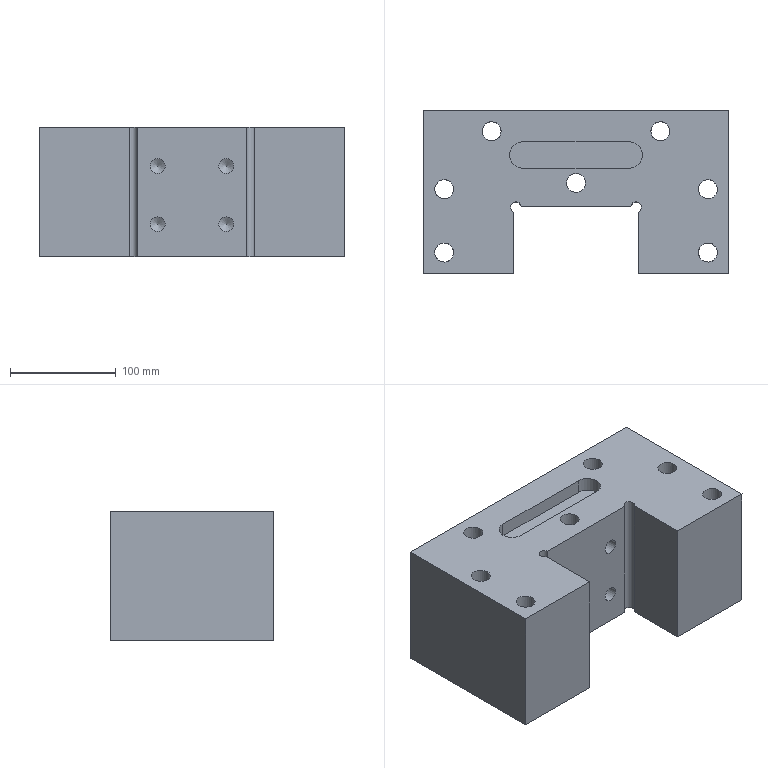Part | STEP file | lll_id778_x_t | 1 solid | 50 faces | box 290 x 155 x 123 mm | volume 4112201 mm3 | cylinder 24 | plane 20 | cone 6 | commonest cylinder face diameters 18.009 x7 26.007 x7 14 x6 10 x2 25 x2
STEP:
#1=CARTESIAN_POINT('',(2079.432,-574.,39.5));
#2=VERTEX_POINT('',#1);
#3=CARTESIAN_POINT('',(2092.435,-574.,39.5));
#4=DIRECTION('',(0.,0.,-1.));
#5=DIRECTION('',(-1.,0.,0.));
#6=AXIS2_PLACEMENT_3D('',#3,#4,#5);
#7=CIRCLE('',#6,13.004);
#8=EDGE_CURVE('',#2,#2,#7,.T.);
#9=ORIENTED_EDGE('',*,*,#8,.F.);
#10=EDGE_LOOP('',(#9));
#11=FACE_BOUND('',#10,.T.);
#12=CARTESIAN_POINT('',(1980.439,-640.,39.5));
#13=VERTEX_POINT('',#12);
#14=CARTESIAN_POINT('',(1967.435,-640.,39.5));
#15=DIRECTION('',(0.,0.,-1.));
#16=DIRECTION('',(1.,0.,0.));
#17=AXIS2_PLACEMENT_3D('',#14,#15,#16);
#18=CIRCLE('',#17,13.004);
#19=EDGE_CURVE('',#13,#13,#18,.T.);
#20=ORIENTED_EDGE('',*,*,#19,.F.);
#21=EDGE_LOOP('',(#20));
#22=FACE_BOUND('',#21,.T.);
#23=CARTESIAN_POINT('',(2230.439,-640.,39.5));
#24=VERTEX_POINT('',#23);
#25=CARTESIAN_POINT('',(2217.435,-640.,39.5));
#26=DIRECTION('',(0.,0.,-1.));
#27=DIRECTION('',(1.,0.,0.));
#28=AXIS2_PLACEMENT_3D('',#25,#26,#27);
#29=CIRCLE('',#28,13.004);
#30=EDGE_CURVE('',#24,#24,#29,.T.);
#31=ORIENTED_EDGE('',*,*,#30,.F.);
#32=EDGE_LOOP('',(#31));
#33=FACE_BOUND('',#32,.T.);
#34=CARTESIAN_POINT('',(1947.435,-660.,39.5));
#35=VERTEX_POINT('',#34);
#36=CARTESIAN_POINT('',(1947.435,-505.,39.5));
#37=VERTEX_POINT('',#36);
#38=CARTESIAN_POINT('',(1947.435,-551.,39.5));
#39=DIRECTION('',(0.,1.,0.));
#40=VECTOR('',#39,1.);
#41=LINE('',#38,#40);
#42=EDGE_CURVE('',#35,#37,#41,.T.);
#43=ORIENTED_EDGE('',*,*,#42,.T.);
#44=CARTESIAN_POINT('',(2237.435,-505.,39.5));
#45=VERTEX_POINT('',#44);
#46=CARTESIAN_POINT('',(2172.935,-505.,39.5));
#47=DIRECTION('',(1.,0.,0.));
#48=VECTOR('',#47,1.);
#49=LINE('',#46,#48);
#50=EDGE_CURVE('',#37,#45,#49,.T.);
#51=ORIENTED_EDGE('',*,*,#50,.T.);
#52=CARTESIAN_POINT('',(2237.435,-660.,39.5));
#53=VERTEX_POINT('',#52);
#54=CARTESIAN_POINT('',(2237.435,-631.,39.5));
#55=DIRECTION('',(0.,-1.,0.));
#56=VECTOR('',#55,1.);
#57=LINE('',#54,#56);
#58=EDGE_CURVE('',#45,#53,#57,.T.);
#59=ORIENTED_EDGE('',*,*,#58,.T.);
#60=CARTESIAN_POINT('',(2151.435,-660.,39.5));
#61=VERTEX_POINT('',#60);
#62=CARTESIAN_POINT('',(2173.935,-660.,39.5));
#63=DIRECTION('',(-1.,0.,0.));
#64=VECTOR('',#63,1.);
#65=LINE('',#62,#64);
#66=EDGE_CURVE('',#53,#61,#65,.T.);
#67=ORIENTED_EDGE('',*,*,#66,.T.);
#68=CARTESIAN_POINT('',(2151.435,-601.583,39.5));
#69=VERTEX_POINT('',#68);
#70=CARTESIAN_POINT('',(2151.435,-574.,39.5));
#71=DIRECTION('',(0.,1.,0.));
#72=VECTOR('',#71,1.);
#73=LINE('',#70,#72);
#74=EDGE_CURVE('',#61,#69,#73,.T.);
#75=ORIENTED_EDGE('',*,*,#74,.T.);
#76=CARTESIAN_POINT('',(2144.536,-596.,39.5));
#77=VERTEX_POINT('',#76);
#78=CARTESIAN_POINT('',(2149.435,-597.,39.5));
#79=DIRECTION('',(0.,0.,1.));
#80=DIRECTION('',(-1.,0.,0.));
#81=AXIS2_PLACEMENT_3D('',#78,#79,#80);
#82=CIRCLE('',#81,5.);
#83=EDGE_CURVE('',#69,#77,#82,.T.);
#84=ORIENTED_EDGE('',*,*,#83,.T.);
#85=CARTESIAN_POINT('',(2040.334,-596.,39.5));
#86=VERTEX_POINT('',#85);
#87=CARTESIAN_POINT('',(2137.864,-596.,39.5));
#88=DIRECTION('',(-1.,0.,0.));
#89=VECTOR('',#88,1.);
#90=LINE('',#87,#89);
#91=EDGE_CURVE('',#77,#86,#90,.T.);
#92=ORIENTED_EDGE('',*,*,#91,.T.);
#93=CARTESIAN_POINT('',(2033.435,-601.583,39.5));
#94=VERTEX_POINT('',#93);
#95=CARTESIAN_POINT('',(2035.435,-597.,39.5));
#96=DIRECTION('',(0.,0.,-1.));
#97=DIRECTION('',(-1.,0.,0.));
#98=AXIS2_PLACEMENT_3D('',#95,#96,#97);
#99=CIRCLE('',#98,5.);
#100=EDGE_CURVE('',#94,#86,#99,.T.);
#101=ORIENTED_EDGE('',*,*,#100,.F.);
#102=CARTESIAN_POINT('',(2033.435,-660.,39.5));
#103=VERTEX_POINT('',#102);
#104=CARTESIAN_POINT('',(2033.435,-631.,39.5));
#105=DIRECTION('',(0.,-1.,0.));
#106=VECTOR('',#105,1.);
#107=LINE('',#104,#106);
#108=EDGE_CURVE('',#94,#103,#107,.T.);
#109=ORIENTED_EDGE('',*,*,#108,.T.);
#110=CARTESIAN_POINT('',(1972.935,-660.,39.5));
#111=DIRECTION('',(-1.,0.,0.));
#112=VECTOR('',#111,1.);
#113=LINE('',#110,#112);
#114=EDGE_CURVE('',#103,#35,#113,.T.);
#115=ORIENTED_EDGE('',*,*,#114,.T.);
#116=EDGE_LOOP('',(#43,#51,#59,#67,#75,#84,#92,#101,#109,#115));
#117=FACE_BOUND('',#116,.T.);
#118=CARTESIAN_POINT('',(1986.436,-603.999,39.5));
#119=VERTEX_POINT('',#118);
#120=CARTESIAN_POINT('',(1993.436,-603.999,39.5));
#121=DIRECTION('',(0.,0.,-1.));
#122=DIRECTION('',(-1.,0.,0.));
#123=AXIS2_PLACEMENT_3D('',#120,#121,#122);
#124=CIRCLE('',#123,7.);
#125=EDGE_CURVE('',#119,#119,#124,.T.);
#126=ORIENTED_EDGE('',*,*,#125,.F.);
#127=EDGE_LOOP('',(#126));
#128=FACE_BOUND('',#127,.T.);
#129=CARTESIAN_POINT('',(2184.434,-603.999,39.5));
#130=VERTEX_POINT('',#129);
#131=CARTESIAN_POINT('',(2191.434,-603.999,39.5));
#132=DIRECTION('',(0.,0.,-1.));
#133=DIRECTION('',(-1.,0.,0.));
#134=AXIS2_PLACEMENT_3D('',#131,#132,#133);
#135=CIRCLE('',#134,7.);
#136=EDGE_CURVE('',#130,#130,#135,.T.);
#137=ORIENTED_EDGE('',*,*,#136,.F.);
#138=EDGE_LOOP('',(#137));
#139=FACE_BOUND('',#138,.T.);
#140=CARTESIAN_POINT('',(2230.439,-580.,39.5));
#141=VERTEX_POINT('',#140);
#142=CARTESIAN_POINT('',(2217.435,-580.,39.5));
#143=DIRECTION('',(0.,0.,-1.));
#144=DIRECTION('',(1.,0.,0.));
#145=AXIS2_PLACEMENT_3D('',#142,#143,#144);
#146=CIRCLE('',#145,13.004);
#147=EDGE_CURVE('',#141,#141,#146,.T.);
#148=ORIENTED_EDGE('',*,*,#147,.F.);
#149=EDGE_LOOP('',(#148));
#150=FACE_BOUND('',#149,.T.);
#151=CARTESIAN_POINT('',(2185.439,-525.,39.5));
#152=VERTEX_POINT('',#151);
#153=CARTESIAN_POINT('',(2172.435,-525.,39.5));
#154=DIRECTION('',(0.,0.,-1.));
#155=DIRECTION('',(1.,0.,0.));
#156=AXIS2_PLACEMENT_3D('',#153,#154,#155);
#157=CIRCLE('',#156,13.004);
#158=EDGE_CURVE('',#152,#152,#157,.T.);
#159=ORIENTED_EDGE('',*,*,#158,.F.);
#160=EDGE_LOOP('',(#159));
#161=FACE_BOUND('',#160,.T.);
#162=CARTESIAN_POINT('',(1980.439,-580.,39.5));
#163=VERTEX_POINT('',#162);
#164=CARTESIAN_POINT('',(1967.435,-580.,39.5));
#165=DIRECTION('',(0.,0.,-1.));
#166=DIRECTION('',(1.,0.,0.));
#167=AXIS2_PLACEMENT_3D('',#164,#165,#166);
#168=CIRCLE('',#167,13.004);
#169=EDGE_CURVE('',#163,#163,#168,.T.);
#170=ORIENTED_EDGE('',*,*,#169,.F.);
#171=EDGE_LOOP('',(#170));
#172=FACE_BOUND('',#171,.T.);
#173=CARTESIAN_POINT('',(1999.432,-525.,39.5));
#174=VERTEX_POINT('',#173);
#175=CARTESIAN_POINT('',(2012.435,-525.,39.5));
#176=DIRECTION('',(0.,0.,1.));
#177=DIRECTION('',(-1.,0.,0.));
#178=AXIS2_PLACEMENT_3D('',#175,#176,#177);
#179=CIRCLE('',#178,13.004);
#180=EDGE_CURVE('',#174,#174,#179,.T.);
#181=ORIENTED_EDGE('',*,*,#180,.T.);
#182=EDGE_LOOP('',(#181));
#183=FACE_BOUND('',#182,.T.);
#184=CARTESIAN_POINT('',(2132.435,0.,39.5));
#185=DIRECTION('',(0.,0.,-1.));
#186=DIRECTION('',(-1.,0.,0.));
#187=AXIS2_PLACEMENT_3D('',#184,#185,#186);
#188=PLANE('',#187);
#189=ADVANCED_FACE('',(#11,#22,#33,#117,#128,#139,#150,#161,#172,#183),#188,.T.);
#190=CARTESIAN_POINT('',(2059.935,-546.,77.5));
#191=VERTEX_POINT('',#190);
#192=CARTESIAN_POINT('',(2059.935,-546.,70.5));
#193=DIRECTION('',(0.,1.,0.000000092));
#194=DIRECTION('',(0.,-0.000000092,1.));
#195=AXIS2_PLACEMENT_3D('',#192,#193,#194);
#196=CIRCLE('',#195,7.);
#197=EDGE_CURVE('',#191,#191,#196,.T.);
#198=ORIENTED_EDGE('',*,*,#197,.F.);
#199=EDGE_LOOP('',(#198));
#200=FACE_BOUND('',#199,.T.);
#201=CARTESIAN_POINT('',(2059.935,-541.794,70.5));
#202=VERTEX_POINT('',#201);
#203=VERTEX_LOOP('',#202);
#204=FACE_BOUND('',#203,.T.);
#205=CARTESIAN_POINT('',(2059.935,-546.,70.5));
#206=DIRECTION('',(0.,-1.,-0.000000092));
#207=DIRECTION('',(0.,0.000000092,-1.));
#208=AXIS2_PLACEMENT_3D('',#205,#206,#207);
#209=CONICAL_SURFACE('',#208,7.,59.);
#210=ADVANCED_FACE('',(#200,#204),#209,.F.);
#211=CARTESIAN_POINT('',(2124.935,-546.,77.5));
#212=VERTEX_POINT('',#211);
#213=CARTESIAN_POINT('',(2124.935,-546.,70.5));
#214=DIRECTION('',(0.,1.,0.000000092));
#215=DIRECTION('',(0.,-0.000000092,1.));
#216=AXIS2_PLACEMENT_3D('',#213,#214,#215);
#217=CIRCLE('',#216,7.);
#218=EDGE_CURVE('',#212,#212,#217,.T.);
#219=ORIENTED_EDGE('',*,*,#218,.F.);
#220=EDGE_LOOP('',(#219));
#221=FACE_BOUND('',#220,.T.);
#222=CARTESIAN_POINT('',(2124.935,-541.794,70.5));
#223=VERTEX_POINT('',#222);
#224=VERTEX_LOOP('',#223);
#225=FACE_BOUND('',#224,.T.);
#226=CARTESIAN_POINT('',(2124.935,-546.,70.5));
#227=DIRECTION('',(0.,-1.,-0.000000092));
#228=DIRECTION('',(0.,0.000000092,-1.));
#229=AXIS2_PLACEMENT_3D('',#226,#227,#228);
#230=CONICAL_SURFACE('',#229,7.,59.);
#231=ADVANCED_FACE('',(#221,#225),#230,.F.);
#232=CARTESIAN_POINT('',(2124.935,-546.,132.5));
#233=VERTEX_POINT('',#232);
#234=CARTESIAN_POINT('',(2124.935,-546.,125.5));
#235=DIRECTION('',(0.,1.,0.000000092));
#236=DIRECTION('',(0.,-0.000000092,1.));
#237=AXIS2_PLACEMENT_3D('',#234,#235,#236);
#238=CIRCLE('',#237,7.);
#239=EDGE_CURVE('',#233,#233,#238,.T.);
#240=ORIENTED_EDGE('',*,*,#239,.F.);
#241=EDGE_LOOP('',(#240));
#242=FACE_BOUND('',#241,.T.);
#243=CARTESIAN_POINT('',(2124.935,-541.794,125.5));
#244=VERTEX_POINT('',#243);
#245=VERTEX_LOOP('',#244);
#246=FACE_BOUND('',#245,.T.);
#247=CARTESIAN_POINT('',(2124.935,-546.,125.5));
#248=DIRECTION('',(0.,-1.,-0.000000092));
#249=DIRECTION('',(0.,0.000000092,-1.));
#250=AXIS2_PLACEMENT_3D('',#247,#248,#249);
#251=CONICAL_SURFACE('',#250,7.,59.);
#252=ADVANCED_FACE('',(#242,#246),#251,.F.);
#253=CARTESIAN_POINT('',(2059.935,-546.,132.5));
#254=VERTEX_POINT('',#253);
#255=CARTESIAN_POINT('',(2059.935,-546.,125.5));
#256=DIRECTION('',(0.,1.,0.000000092));
#257=DIRECTION('',(0.,-0.000000092,1.));
#258=AXIS2_PLACEMENT_3D('',#255,#256,#257);
#259=CIRCLE('',#258,7.);
#260=EDGE_CURVE('',#254,#254,#259,.T.);
#261=ORIENTED_EDGE('',*,*,#260,.F.);
#262=EDGE_LOOP('',(#261));
#263=FACE_BOUND('',#262,.T.);
#264=CARTESIAN_POINT('',(2059.935,-541.794,125.5));
#265=VERTEX_POINT('',#264);
#266=VERTEX_LOOP('',#265);
#267=FACE_BOUND('',#266,.T.);
#268=CARTESIAN_POINT('',(2059.935,-546.,125.5));
#269=DIRECTION('',(0.,-1.,-0.000000092));
#270=DIRECTION('',(0.,0.000000092,-1.));
#271=AXIS2_PLACEMENT_3D('',#268,#269,#270);
#272=CONICAL_SURFACE('',#271,7.,59.);
#273=ADVANCED_FACE('',(#263,#267),#272,.F.);
#274=CARTESIAN_POINT('',(1993.436,-596.999,119.449));
#275=VERTEX_POINT('',#274);
#276=CARTESIAN_POINT('',(1993.436,-603.999,119.449));
#277=DIRECTION('',(0.,-0.000000092,1.));
#278=DIRECTION('',(0.,1.,0.000000092));
#279=AXIS2_PLACEMENT_3D('',#276,#277,#278);
#280=CIRCLE('',#279,7.);
#281=EDGE_CURVE('',#275,#275,#280,.T.);
#282=ORIENTED_EDGE('',*,*,#281,.F.);
#283=EDGE_LOOP('',(#282));
#284=FACE_BOUND('',#283,.T.);
#285=CARTESIAN_POINT('',(1993.436,-603.999,123.655));
#286=VERTEX_POINT('',#285);
#287=VERTEX_LOOP('',#286);
#288=FACE_BOUND('',#287,.T.);
#289=CARTESIAN_POINT('',(1993.436,-603.999,120.5));
#290=DIRECTION('',(0.,0.000000092,-1.));
#291=DIRECTION('',(0.,1.,0.000000092));
#292=AXIS2_PLACEMENT_3D('',#289,#290,#291);
#293=CONICAL_SURFACE('',#292,5.25,59.);
#294=ADVANCED_FACE('',(#284,#288),#293,.F.);
#295=ORIENTED_EDGE('',*,*,#197,.T.);
#296=EDGE_LOOP('',(#295));
#297=FACE_BOUND('',#296,.T.);
#298=CARTESIAN_POINT('',(2059.935,-596.,77.5));
#299=VERTEX_POINT('',#298);
#300=CARTESIAN_POINT('',(2059.935,-596.,70.5));
#301=DIRECTION('',(0.,-1.,-0.000000092));
#302=DIRECTION('',(0.,-0.000000092,1.));
#303=AXIS2_PLACEMENT_3D('',#300,#301,#302);
#304=CIRCLE('',#303,7.);
#305=EDGE_CURVE('',#299,#299,#304,.T.);
#306=ORIENTED_EDGE('',*,*,#305,.T.);
#307=EDGE_LOOP('',(#306));
#308=FACE_BOUND('',#307,.T.);
#309=CARTESIAN_POINT('',(2059.935,-596.,70.5));
#310=DIRECTION('',(0.,1.,0.000000092));
#311=DIRECTION('',(0.,-0.000000092,1.));
#312=AXIS2_PLACEMENT_3D('',#309,#310,#311);
#313=CYLINDRICAL_SURFACE('',#312,7.);
#314=ADVANCED_FACE('',(#297,#308),#313,.F.);
#315=ORIENTED_EDGE('',*,*,#218,.T.);
#316=EDGE_LOOP('',(#315));
#317=FACE_BOUND('',#316,.T.);
#318=CARTESIAN_POINT('',(2124.935,-596.,77.5));
#319=VERTEX_POINT('',#318);
#320=CARTESIAN_POINT('',(2124.935,-596.,70.5));
#321=DIRECTION('',(0.,-1.,-0.000000092));
#322=DIRECTION('',(0.,-0.000000092,1.));
#323=AXIS2_PLACEMENT_3D('',#320,#321,#322);
#324=CIRCLE('',#323,7.);
#325=EDGE_CURVE('',#319,#319,#324,.T.);
#326=ORIENTED_EDGE('',*,*,#325,.T.);
#327=EDGE_LOOP('',(#326));
#328=FACE_BOUND('',#327,.T.);
#329=CARTESIAN_POINT('',(2124.935,-596.,70.5));
#330=DIRECTION('',(0.,1.,0.000000092));
#331=DIRECTION('',(0.,-0.000000092,1.));
#332=AXIS2_PLACEMENT_3D('',#329,#330,#331);
#333=CYLINDRICAL_SURFACE('',#332,7.);
#334=ADVANCED_FACE('',(#317,#328),#333,.F.);
#335=ORIENTED_EDGE('',*,*,#239,.T.);
#336=EDGE_LOOP('',(#335));
#337=FACE_BOUND('',#336,.T.);
#338=CARTESIAN_POINT('',(2124.935,-596.,132.5));
#339=VERTEX_POINT('',#338);
#340=CARTESIAN_POINT('',(2124.935,-596.,125.5));
#341=DIRECTION('',(0.,-1.,-0.000000092));
#342=DIRECTION('',(0.,-0.000000092,1.));
#343=AXIS2_PLACEMENT_3D('',#340,#341,#342);
#344=CIRCLE('',#343,7.);
#345=EDGE_CURVE('',#339,#339,#344,.T.);
#346=ORIENTED_EDGE('',*,*,#345,.T.);
#347=EDGE_LOOP('',(#346));
#348=FACE_BOUND('',#347,.T.);
#349=CARTESIAN_POINT('',(2124.935,-596.,125.5));
#350=DIRECTION('',(0.,1.,0.000000092));
#351=DIRECTION('',(0.,-0.000000092,1.));
#352=AXIS2_PLACEMENT_3D('',#349,#350,#351);
#353=CYLINDRICAL_SURFACE('',#352,7.);
#354=ADVANCED_FACE('',(#337,#348),#353,.F.);
#355=ORIENTED_EDGE('',*,*,#260,.T.);
#356=EDGE_LOOP('',(#355));
#357=FACE_BOUND('',#356,.T.);
#358=CARTESIAN_POINT('',(2059.935,-596.,132.5));
#359=VERTEX_POINT('',#358);
#360=CARTESIAN_POINT('',(2059.935,-596.,125.5));
#361=DIRECTION('',(0.,-1.,-0.000000092));
#362=DIRECTION('',(0.,-0.000000092,1.));
#363=AXIS2_PLACEMENT_3D('',#360,#361,#362);
#364=CIRCLE('',#363,7.);
#365=EDGE_CURVE('',#359,#359,#364,.T.);
#366=ORIENTED_EDGE('',*,*,#365,.T.);
#367=EDGE_LOOP('',(#366));
#368=FACE_BOUND('',#367,.T.);
#369=CARTESIAN_POINT('',(2059.935,-596.,125.5));
#370=DIRECTION('',(0.,1.,0.000000092));
#371=DIRECTION('',(0.,-0.000000092,1.));
#372=AXIS2_PLACEMENT_3D('',#369,#370,#371);
#373=CYLINDRICAL_SURFACE('',#372,7.);
#374=ADVANCED_FACE('',(#357,#368),#373,.F.);
#375=ORIENTED_EDGE('',*,*,#281,.T.);
#376=EDGE_LOOP('',(#375));
#377=FACE_BOUND('',#376,.T.);
#378=ORIENTED_EDGE('',*,*,#125,.T.);
#379=EDGE_LOOP('',(#378));
#380=FACE_BOUND('',#379,.T.);
#381=CARTESIAN_POINT('',(1993.436,-603.999,110.5));
#382=DIRECTION('',(0.,-0.000000092,1.));
#383=DIRECTION('',(0.,-1.,-0.000000092));
#384=AXIS2_PLACEMENT_3D('',#381,#382,#383);
#385=CYLINDRICAL_SURFACE('',#384,7.);
#386=ADVANCED_FACE('',(#377,#380),#385,.F.);
#387=CARTESIAN_POINT('',(1947.435,-505.,162.5));
#388=VERTEX_POINT('',#387);
#389=CARTESIAN_POINT('',(1947.435,-660.,162.5));
#390=VERTEX_POINT('',#389);
#391=CARTESIAN_POINT('',(1947.435,-574.,162.5));
#392=DIRECTION('',(0.,-1.,-0.000000092));
#393=VECTOR('',#392,1.);
#394=LINE('',#391,#393);
#395=EDGE_CURVE('',#388,#390,#394,.T.);
#396=ORIENTED_EDGE('',*,*,#395,.F.);
#397=CARTESIAN_POINT('',(1947.435,-505.,76.5));
#398=DIRECTION('',(0.,0.000000092,-1.));
#399=VECTOR('',#398,1.);
#400=LINE('',#397,#399);
#401=EDGE_CURVE('',#388,#37,#400,.T.);
#402=ORIENTED_EDGE('',*,*,#401,.T.);
#403=ORIENTED_EDGE('',*,*,#42,.F.);
#404=CARTESIAN_POINT('',(1947.435,-660.,76.5));
#405=DIRECTION('',(0.,0.000000092,-1.));
#406=VECTOR('',#405,1.);
#407=LINE('',#404,#406);
#408=EDGE_CURVE('',#390,#35,#407,.T.);
#409=ORIENTED_EDGE('',*,*,#408,.F.);
#410=EDGE_LOOP('',(#396,#402,#403,#409));
#411=FACE_OUTER_BOUND('',#410,.T.);
#412=CARTESIAN_POINT('',(1947.435,-551.,76.5));
#413=DIRECTION('',(1.,0.,0.));
#414=DIRECTION('',(0.,0.000000092,-1.));
#415=AXIS2_PLACEMENT_3D('',#412,#413,#414);
#416=PLANE('',#415);
#417=ADVANCED_FACE('',(#411),#416,.F.);
#418=CARTESIAN_POINT('',(2033.435,-660.,162.5));
#419=VERTEX_POINT('',#418);
#420=CARTESIAN_POINT('',(1972.935,-660.,162.5));
#421=DIRECTION('',(-1.,0.,0.));
#422=VECTOR('',#421,1.);
#423=LINE('',#420,#422);
#424=EDGE_CURVE('',#419,#390,#423,.T.);
#425=ORIENTED_EDGE('',*,*,#424,.T.);
#426=ORIENTED_EDGE('',*,*,#408,.T.);
#427=ORIENTED_EDGE('',*,*,#114,.F.);
#428=CARTESIAN_POINT('',(2033.435,-660.,76.5));
#429=DIRECTION('',(0.,0.000000092,-1.));
#430=VECTOR('',#429,1.);
#431=LINE('',#428,#430);
#432=EDGE_CURVE('',#419,#103,#431,.T.);
#433=ORIENTED_EDGE('',*,*,#432,.F.);
#434=EDGE_LOOP('',(#425,#426,#427,#433));
#435=FACE_OUTER_BOUND('',#434,.T.);
#436=CARTESIAN_POINT('',(1972.935,-660.,76.5));
#437=DIRECTION('',(0.,1.,0.000000092));
#438=DIRECTION('',(-1.,0.,0.));
#439=AXIS2_PLACEMENT_3D('',#436,#437,#438);
#440=PLANE('',#439);
#441=ADVANCED_FACE('',(#435),#440,.F.);
#442=CARTESIAN_POINT('',(2033.435,-601.583,162.5));
#443=VERTEX_POINT('',#442);
#444=CARTESIAN_POINT('',(2033.435,-631.,162.5));
#445=DIRECTION('',(0.,-1.,-0.000000092));
#446=VECTOR('',#445,1.);
#447=LINE('',#444,#446);
#448=EDGE_CURVE('',#443,#419,#447,.T.);
#449=ORIENTED_EDGE('',*,*,#448,.T.);
#450=ORIENTED_EDGE('',*,*,#432,.T.);
#451=ORIENTED_EDGE('',*,*,#108,.F.);
#452=CARTESIAN_POINT('',(2033.435,-601.583,180.5));
#453=DIRECTION('',(0.,0.000000092,-1.));
#454=VECTOR('',#453,1.);
#455=LINE('',#452,#454);
#456=EDGE_CURVE('',#443,#94,#455,.T.);
#457=ORIENTED_EDGE('',*,*,#456,.F.);
#458=EDGE_LOOP('',(#449,#450,#451,#457));
#459=FACE_OUTER_BOUND('',#458,.T.);
#460=CARTESIAN_POINT('',(2033.435,-631.,76.5));
#461=DIRECTION('',(-1.,0.,0.));
#462=DIRECTION('',(0.,-0.000000092,1.));
#463=AXIS2_PLACEMENT_3D('',#460,#461,#462);
#464=PLANE('',#463);
#465=ADVANCED_FACE('',(#459),#464,.F.);
#466=ORIENTED_EDGE('',*,*,#100,.T.);
#467=CARTESIAN_POINT('',(2040.334,-596.,162.5));
#468=VERTEX_POINT('',#467);
#469=CARTESIAN_POINT('',(2040.334,-596.,100.5));
#470=DIRECTION('',(0.,-0.000000092,1.));
#471=VECTOR('',#470,1.);
#472=LINE('',#469,#471);
#473=EDGE_CURVE('',#86,#468,#472,.T.);
#474=ORIENTED_EDGE('',*,*,#473,.T.);
#475=CARTESIAN_POINT('',(2035.435,-597.,162.5));
#476=DIRECTION('',(0.,0.000000092,-1.));
#477=DIRECTION('',(0.,1.,0.000000092));
#478=AXIS2_PLACEMENT_3D('',#475,#476,#477);
#479=CIRCLE('',#478,5.);
#480=EDGE_CURVE('',#443,#468,#479,.T.);
#481=ORIENTED_EDGE('',*,*,#480,.F.);
#482=ORIENTED_EDGE('',*,*,#456,.T.);
#483=EDGE_LOOP('',(#466,#474,#481,#482));
#484=FACE_OUTER_BOUND('',#483,.T.);
#485=CARTESIAN_POINT('',(2035.435,-597.,80.5));
#486=DIRECTION('',(0.,-0.000000092,1.));
#487=DIRECTION('',(-1.,0.,0.));
#488=AXIS2_PLACEMENT_3D('',#485,#486,#487);
#489=CYLINDRICAL_SURFACE('',#488,5.);
#490=ADVANCED_FACE('',(#484),#489,.F.);
#491=ORIENTED_EDGE('',*,*,#365,.F.);
#492=EDGE_LOOP('',(#491));
#493=FACE_BOUND('',#492,.T.);
#494=ORIENTED_EDGE('',*,*,#345,.F.);
#495=EDGE_LOOP('',(#494));
#496=FACE_BOUND('',#495,.T.);
#497=ORIENTED_EDGE('',*,*,#325,.F.);
#498=EDGE_LOOP('',(#497));
#499=FACE_BOUND('',#498,.T.);
#500=ORIENTED_EDGE('',*,*,#305,.F.);
#501=EDGE_LOOP('',(#500));
#502=FACE_BOUND('',#501,.T.);
#503=ORIENTED_EDGE('',*,*,#91,.F.);
#504=CARTESIAN_POINT('',(2144.536,-596.,162.5));
#505=VERTEX_POINT('',#504);
#506=CARTESIAN_POINT('',(2144.536,-596.,100.5));
#507=DIRECTION('',(0.,-0.000000092,1.));
#508=VECTOR('',#507,1.);
#509=LINE('',#506,#508);
#510=EDGE_CURVE('',#77,#505,#509,.T.);
#511=ORIENTED_EDGE('',*,*,#510,.T.);
#512=CARTESIAN_POINT('',(2137.864,-596.,162.5));
#513=DIRECTION('',(-1.,0.,0.));
#514=VECTOR('',#513,1.);
#515=LINE('',#512,#514);
#516=EDGE_CURVE('',#505,#468,#515,.T.);
#517=ORIENTED_EDGE('',*,*,#516,.T.);
#518=ORIENTED_EDGE('',*,*,#473,.F.);
#519=EDGE_LOOP('',(#503,#511,#517,#518));
#520=FACE_BOUND('',#519,.T.);
#521=CARTESIAN_POINT('',(2137.864,-596.,226.5));
#522=DIRECTION('',(0.,-1.,-0.000000092));
#523=DIRECTION('',(0.,-0.000000092,1.));
#524=AXIS2_PLACEMENT_3D('',#521,#522,#523);
#525=PLANE('',#524);
#526=ADVANCED_FACE('',(#493,#496,#499,#502,#520),#525,.T.);
#527=ORIENTED_EDGE('',*,*,#510,.F.);
#528=ORIENTED_EDGE('',*,*,#83,.F.);
#529=CARTESIAN_POINT('',(2151.435,-601.583,162.5));
#530=VERTEX_POINT('',#529);
#531=CARTESIAN_POINT('',(2151.435,-601.583,180.5));
#532=DIRECTION('',(0.,0.000000092,-1.));
#533=VECTOR('',#532,1.);
#534=LINE('',#531,#533);
#535=EDGE_CURVE('',#530,#69,#534,.T.);
#536=ORIENTED_EDGE('',*,*,#535,.F.);
#537=CARTESIAN_POINT('',(2149.435,-597.,162.5));
#538=DIRECTION('',(0.,-0.000000092,1.));
#539=DIRECTION('',(0.,1.,0.000000092));
#540=AXIS2_PLACEMENT_3D('',#537,#538,#539);
#541=CIRCLE('',#540,5.);
#542=EDGE_CURVE('',#530,#505,#541,.T.);
#543=ORIENTED_EDGE('',*,*,#542,.T.);
#544=EDGE_LOOP('',(#527,#528,#536,#543));
#545=FACE_OUTER_BOUND('',#544,.T.);
#546=CARTESIAN_POINT('',(2149.435,-597.,80.5));
#547=DIRECTION('',(0.,-0.000000092,1.));
#548=DIRECTION('',(-1.,0.,0.));
#549=AXIS2_PLACEMENT_3D('',#546,#547,#548);
#550=CYLINDRICAL_SURFACE('',#549,5.);
#551=ADVANCED_FACE('',(#545),#550,.F.);
#552=ORIENTED_EDGE('',*,*,#535,.T.);
#553=ORIENTED_EDGE('',*,*,#74,.F.);
#554=CARTESIAN_POINT('',(2151.435,-660.,162.5));
#555=VERTEX_POINT('',#554);
#556=CARTESIAN_POINT('',(2151.435,-660.,76.5));
#557=DIRECTION('',(0.,0.000000092,-1.));
#558=VECTOR('',#557,1.);
#559=LINE('',#556,#558);
#560=EDGE_CURVE('',#555,#61,#559,.T.);
#561=ORIENTED_EDGE('',*,*,#560,.F.);
#562=CARTESIAN_POINT('',(2151.435,-574.,162.5));
#563=DIRECTION('',(0.,1.,0.000000092));
#564=VECTOR('',#563,1.);
#565=LINE('',#562,#564);
#566=EDGE_CURVE('',#555,#530,#565,.T.);
#567=ORIENTED_EDGE('',*,*,#566,.T.);
#568=EDGE_LOOP('',(#552,#553,#561,#567));
#569=FACE_OUTER_BOUND('',#568,.T.);
#570=CARTESIAN_POINT('',(2151.435,-574.,76.5));
#571=DIRECTION('',(1.,0.,0.));
#572=DIRECTION('',(0.,0.000000092,-1.));
#573=AXIS2_PLACEMENT_3D('',#570,#571,#572);
#574=PLANE('',#573);
#575=ADVANCED_FACE('',(#569),#574,.F.);
#576=CARTESIAN_POINT('',(2237.435,-660.,162.5));
#577=VERTEX_POINT('',#576);
#578=CARTESIAN_POINT('',(2173.935,-660.,162.5));
#579=DIRECTION('',(-1.,0.,0.));
#580=VECTOR('',#579,1.);
#581=LINE('',#578,#580);
#582=EDGE_CURVE('',#577,#555,#581,.T.);
#583=ORIENTED_EDGE('',*,*,#582,.T.);
#584=ORIENTED_EDGE('',*,*,#560,.T.);
#585=ORIENTED_EDGE('',*,*,#66,.F.);
#586=CARTESIAN_POINT('',(2237.435,-660.,76.5));
#587=DIRECTION('',(0.,0.000000092,-1.));
#588=VECTOR('',#587,1.);
#589=LINE('',#586,#588);
#590=EDGE_CURVE('',#577,#53,#589,.T.);
#591=ORIENTED_EDGE('',*,*,#590,.F.);
#592=EDGE_LOOP('',(#583,#584,#585,#591));
#593=FACE_OUTER_BOUND('',#592,.T.);
#594=CARTESIAN_POINT('',(2173.935,-660.,76.5));
#595=DIRECTION('',(0.,1.,0.000000092));
#596=DIRECTION('',(0.,-0.000000092,1.));
#597=AXIS2_PLACEMENT_3D('',#594,#595,#596);
#598=PLANE('',#597);
#599=ADVANCED_FACE('',(#593),#598,.F.);
#600=ORIENTED_EDGE('',*,*,#58,.F.);
#601=CARTESIAN_POINT('',(2237.435,-505.,162.5));
#602=VERTEX_POINT('',#601);
#603=CARTESIAN_POINT('',(2237.435,-505.,76.5));
#604=DIRECTION('',(0.,0.000000092,-1.));
#605=VECTOR('',#604,1.);
#606=LINE('',#603,#605);
#607=EDGE_CURVE('',#602,#45,#606,.T.);
#608=ORIENTED_EDGE('',*,*,#607,.F.);
#609=CARTESIAN_POINT('',(2237.435,-574.,162.5));
#610=DIRECTION('',(0.,1.,0.000000092));
#611=VECTOR('',#610,1.);
#612=LINE('',#609,#611);
#613=EDGE_CURVE('',#577,#602,#612,.T.);
#614=ORIENTED_EDGE('',*,*,#613,.F.);
#615=ORIENTED_EDGE('',*,*,#590,.T.);
#616=EDGE_LOOP('',(#600,#608,#614,#615));
#617=FACE_OUTER_BOUND('',#616,.T.);
#618=CARTESIAN_POINT('',(2237.435,-631.,76.5));
#619=DIRECTION('',(-1.,0.,0.));
#620=DIRECTION('',(0.,-0.000000092,1.));
#621=AXIS2_PLACEMENT_3D('',#618,#619,#620);
#622=PLANE('',#621);
#623=ADVANCED_FACE('',(#617),#622,.F.);
#624=ORIENTED_EDGE('',*,*,#50,.F.);
#625=ORIENTED_EDGE('',*,*,#401,.F.);
#626=CARTESIAN_POINT('',(2172.935,-505.,162.5));
#627=DIRECTION('',(1.,0.,0.));
#628=VECTOR('',#627,1.);
#629=LINE('',#626,#628);
#630=EDGE_CURVE('',#388,#602,#629,.T.);
#631=ORIENTED_EDGE('',*,*,#630,.T.);
#632=ORIENTED_EDGE('',*,*,#607,.T.);
#633=EDGE_LOOP('',(#624,#625,#631,#632));
#634=FACE_OUTER_BOUND('',#633,.T.);
#635=CARTESIAN_POINT('',(2172.935,-505.,76.5));
#636=DIRECTION('',(0.,-1.,-0.000000092));
#637=DIRECTION('',(0.,0.000000092,-1.));
#638=AXIS2_PLACEMENT_3D('',#635,#636,#637);
#639=PLANE('',#638);
#640=ADVANCED_FACE('',(#634),#639,.F.);
#641=CARTESIAN_POINT('',(2092.435,-564.995,162.5));
#642=VERTEX_POINT('',#641);
#643=CARTESIAN_POINT('',(2092.435,-574.,162.5));
#644=DIRECTION('',(0.,-0.000000092,1.));
#645=DIRECTION('',(0.,1.,0.000000092));
#646=AXIS2_PLACEMENT_3D('',#643,#644,#645);
#647=CIRCLE('',#646,9.005);
#648=EDGE_CURVE('',#642,#642,#647,.T.);
#649=ORIENTED_EDGE('',*,*,#648,.F.);
#650=EDGE_LOOP('',(#649));
#651=FACE_BOUND('',#650,.T.);
#652=CARTESIAN_POINT('',(2041.935,-560.,162.5));
#653=VERTEX_POINT('',#652);
#654=CARTESIAN_POINT('',(2041.935,-535.,162.5));
#655=VERTEX_POINT('',#654);
#656=CARTESIAN_POINT('',(2041.935,-547.5,162.5));
#657=DIRECTION('',(0.,0.000000092,-1.));
#658=DIRECTION('',(0.,1.,0.000000092));
#659=AXIS2_PLACEMENT_3D('',#656,#657,#658);
#660=CIRCLE('',#659,12.5);
#661=EDGE_CURVE('',#653,#655,#660,.T.);
#662=ORIENTED_EDGE('',*,*,#661,.T.);
#663=CARTESIAN_POINT('',(2142.935,-535.,162.5));
#664=VERTEX_POINT('',#663);
#665=CARTESIAN_POINT('',(2034.935,-535.,162.5));
#666=DIRECTION('',(1.,0.,0.));
#667=VECTOR('',#666,1.);
#668=LINE('',#665,#667);
#669=EDGE_CURVE('',#655,#664,#668,.T.);
#670=ORIENTED_EDGE('',*,*,#669,.T.);
#671=CARTESIAN_POINT('',(2142.935,-560.,162.5));
#672=VERTEX_POINT('',#671);
#673=CARTESIAN_POINT('',(2142.935,-547.5,162.5));
#674=DIRECTION('',(0.,0.000000092,-1.));
#675=DIRECTION('',(0.,1.,0.000000092));
#676=AXIS2_PLACEMENT_3D('',#673,#674,#675);
#677=CIRCLE('',#676,12.5);
#678=EDGE_CURVE('',#664,#672,#677,.T.);
#679=ORIENTED_EDGE('',*,*,#678,.T.);
#680=CARTESIAN_POINT('',(2034.935,-560.,162.5));
#681=DIRECTION('',(-1.,0.,0.));
#682=VECTOR('',#681,1.);
#683=LINE('',#680,#682);
#684=EDGE_CURVE('',#672,#653,#683,.T.);
#685=ORIENTED_EDGE('',*,*,#684,.T.);
#686=EDGE_LOOP('',(#662,#670,#679,#685));
#687=FACE_BOUND('',#686,.T.);
#688=CARTESIAN_POINT('',(1967.435,-630.996,162.5));
#689=VERTEX_POINT('',#688);
#690=CARTESIAN_POINT('',(1967.435,-640.,162.5));
#691=DIRECTION('',(0.,0.000000092,-1.));
#692=DIRECTION('',(0.,1.,0.000000092));
#693=AXIS2_PLACEMENT_3D('',#690,#691,#692);
#694=CIRCLE('',#693,9.005);
#695=EDGE_CURVE('',#689,#689,#694,.T.);
#696=ORIENTED_EDGE('',*,*,#695,.T.);
#697=EDGE_LOOP('',(#696));
#698=FACE_BOUND('',#697,.T.);
#699=CARTESIAN_POINT('',(2217.435,-630.996,162.5));
#700=VERTEX_POINT('',#699);
#701=CARTESIAN_POINT('',(2217.435,-640.,162.5));
#702=DIRECTION('',(0.,0.000000092,-1.));
#703=DIRECTION('',(0.,1.,0.000000092));
#704=AXIS2_PLACEMENT_3D('',#701,#702,#703);
#705=CIRCLE('',#704,9.005);
#706=EDGE_CURVE('',#700,#700,#705,.T.);
#707=ORIENTED_EDGE('',*,*,#706,.T.);
#708=EDGE_LOOP('',(#707));
#709=FACE_BOUND('',#708,.T.);
#710=CARTESIAN_POINT('',(2012.435,-515.995,162.5));
#711=VERTEX_POINT('',#710);
#712=CARTESIAN_POINT('',(2012.435,-525.,162.5));
#713=DIRECTION('',(0.,0.000000092,-1.));
#714=DIRECTION('',(0.,1.,0.000000092));
#715=AXIS2_PLACEMENT_3D('',#712,#713,#714);
#716=CIRCLE('',#715,9.005);
#717=EDGE_CURVE('',#711,#711,#716,.T.);
#718=ORIENTED_EDGE('',*,*,#717,.T.);
#719=EDGE_LOOP('',(#718));
#720=FACE_BOUND('',#719,.T.);
#721=CARTESIAN_POINT('',(1967.435,-570.995,162.5));
#722=VERTEX_POINT('',#721);
#723=CARTESIAN_POINT('',(1967.435,-580.,162.5));
#724=DIRECTION('',(0.,0.000000092,-1.));
#725=DIRECTION('',(0.,1.,0.000000092));
#726=AXIS2_PLACEMENT_3D('',#723,#724,#725);
#727=CIRCLE('',#726,9.005);
#728=EDGE_CURVE('',#722,#722,#727,.T.);
#729=ORIENTED_EDGE('',*,*,#728,.T.);
#730=EDGE_LOOP('',(#729));
#731=FACE_BOUND('',#730,.T.);
#732=CARTESIAN_POINT('',(2172.435,-515.995,162.5));
#733=VERTEX_POINT('',#732);
#734=CARTESIAN_POINT('',(2172.435,-525.,162.5));
#735=DIRECTION('',(0.,0.000000092,-1.));
#736=DIRECTION('',(0.,1.,0.000000092));
#737=AXIS2_PLACEMENT_3D('',#734,#735,#736);
#738=CIRCLE('',#737,9.005);
#739=EDGE_CURVE('',#733,#733,#738,.T.);
#740=ORIENTED_EDGE('',*,*,#739,.T.);
#741=EDGE_LOOP('',(#740));
#742=FACE_BOUND('',#741,.T.);
#743=CARTESIAN_POINT('',(2217.435,-570.995,162.5));
#744=VERTEX_POINT('',#743);
#745=CARTESIAN_POINT('',(2217.435,-580.,162.5));
#746=DIRECTION('',(0.,0.000000092,-1.));
#747=DIRECTION('',(0.,1.,0.000000092));
#748=AXIS2_PLACEMENT_3D('',#745,#746,#747);
#749=CIRCLE('',#748,9.005);
#750=EDGE_CURVE('',#744,#744,#749,.T.);
#751=ORIENTED_EDGE('',*,*,#750,.T.);
#752=EDGE_LOOP('',(#751));
#753=FACE_BOUND('',#752,.T.);
#754=ORIENTED_EDGE('',*,*,#630,.F.);
#755=ORIENTED_EDGE('',*,*,#395,.T.);
#756=ORIENTED_EDGE('',*,*,#424,.F.);
#757=ORIENTED_EDGE('',*,*,#448,.F.);
#758=ORIENTED_EDGE('',*,*,#480,.T.);
#759=ORIENTED_EDGE('',*,*,#516,.F.);
#760=ORIENTED_EDGE('',*,*,#542,.F.);
#761=ORIENTED_EDGE('',*,*,#566,.F.);
#762=ORIENTED_EDGE('',*,*,#582,.F.);
#763=ORIENTED_EDGE('',*,*,#613,.T.);
#764=EDGE_LOOP('',(#754,#755,#756,#757,#758,#759,#760,#761,#762,#763));
#765=FACE_BOUND('',#764,.T.);
#766=CARTESIAN_POINT('',(2034.935,-574.,162.5));
#767=DIRECTION('',(0.,-0.000000092,1.));
#768=DIRECTION('',(1.,0.,0.));
#769=AXIS2_PLACEMENT_3D('',#766,#767,#768);
#770=PLANE('',#769);
#771=ADVANCED_FACE('',(#651,#687,#698,#709,#720,#731,#742,#753,#765),#770,.T.);
#772=CARTESIAN_POINT('',(2191.434,-596.999,119.449));
#773=VERTEX_POINT('',#772);
#774=CARTESIAN_POINT('',(2191.434,-603.999,119.449));
#775=DIRECTION('',(0.,-0.000000092,1.));
#776=DIRECTION('',(0.,1.,0.000000092));
#777=AXIS2_PLACEMENT_3D('',#774,#775,#776);
#778=CIRCLE('',#777,7.);
#779=EDGE_CURVE('',#773,#773,#778,.T.);
#780=ORIENTED_EDGE('',*,*,#779,.F.);
#781=EDGE_LOOP('',(#780));
#782=FACE_BOUND('',#781,.T.);
#783=CARTESIAN_POINT('',(2191.434,-603.999,123.655));
#784=VERTEX_POINT('',#783);
#785=VERTEX_LOOP('',#784);
#786=FACE_BOUND('',#785,.T.);
#787=CARTESIAN_POINT('',(2191.434,-603.999,120.5));
#788=DIRECTION('',(0.,0.000000092,-1.));
#789=DIRECTION('',(0.,1.,0.000000092));
#790=AXIS2_PLACEMENT_3D('',#787,#788,#789);
#791=CONICAL_SURFACE('',#790,5.25,59.);
#792=ADVANCED_FACE('',(#782,#786),#791,.F.);
#793=ORIENTED_EDGE('',*,*,#779,.T.);
#794=EDGE_LOOP('',(#793));
#795=FACE_BOUND('',#794,.T.);
#796=ORIENTED_EDGE('',*,*,#136,.T.);
#797=EDGE_LOOP('',(#796));
#798=FACE_BOUND('',#797,.T.);
#799=CARTESIAN_POINT('',(2191.434,-603.999,110.5));
#800=DIRECTION('',(0.,-0.000000092,1.));
#801=DIRECTION('',(0.,-1.,-0.000000092));
#802=AXIS2_PLACEMENT_3D('',#799,#800,#801);
#803=CYLINDRICAL_SURFACE('',#802,7.);
#804=ADVANCED_FACE('',(#795,#798),#803,.F.);
#805=ORIENTED_EDGE('',*,*,#750,.F.);
#806=EDGE_LOOP('',(#805));
#807=FACE_BOUND('',#806,.T.);
#808=CARTESIAN_POINT('',(2226.44,-580.,122.5));
#809=VERTEX_POINT('',#808);
#810=CARTESIAN_POINT('',(2217.435,-580.,122.5));
#811=DIRECTION('',(0.,0.,-1.));
#812=DIRECTION('',(1.,0.,0.));
#813=AXIS2_PLACEMENT_3D('',#810,#811,#812);
#814=CIRCLE('',#813,9.005);
#815=EDGE_CURVE('',#809,#809,#814,.T.);
#816=ORIENTED_EDGE('',*,*,#815,.T.);
#817=EDGE_LOOP('',(#816));
#818=FACE_BOUND('',#817,.T.);
#819=CARTESIAN_POINT('',(2217.435,-580.,34.5));
#820=DIRECTION('',(0.,0.,1.));
#821=DIRECTION('',(1.,0.,0.));
#822=AXIS2_PLACEMENT_3D('',#819,#820,#821);
#823=CYLINDRICAL_SURFACE('',#822,9.005);
#824=ADVANCED_FACE('',(#807,#818),#823,.F.);
#825=ORIENTED_EDGE('',*,*,#815,.F.);
#826=EDGE_LOOP('',(#825));
#827=FACE_BOUND('',#826,.T.);
#828=CARTESIAN_POINT('',(2230.439,-580.,122.5));
#829=VERTEX_POINT('',#828);
#830=CARTESIAN_POINT('',(2217.435,-580.,122.5));
#831=DIRECTION('',(0.,0.,-1.));
#832=DIRECTION('',(1.,0.,0.));
#833=AXIS2_PLACEMENT_3D('',#830,#831,#832);
#834=CIRCLE('',#833,13.004);
#835=EDGE_CURVE('',#829,#829,#834,.T.);
#836=ORIENTED_EDGE('',*,*,#835,.T.);
#837=EDGE_LOOP('',(#836));
#838=FACE_BOUND('',#837,.T.);
#839=CARTESIAN_POINT('',(2217.435,-580.,122.5));
#840=DIRECTION('',(0.,0.,1.));
#841=DIRECTION('',(1.,0.,0.));
#842=AXIS2_PLACEMENT_3D('',#839,#840,#841);
#843=PLANE('',#842);
#844=ADVANCED_FACE('',(#827,#838),#843,.F.);
#845=ORIENTED_EDGE('',*,*,#835,.F.);
#846=EDGE_LOOP('',(#845));
#847=FACE_BOUND('',#846,.T.);
#848=ORIENTED_EDGE('',*,*,#147,.T.);
#849=EDGE_LOOP('',(#848));
#850=FACE_BOUND('',#849,.T.);
#851=CARTESIAN_POINT('',(2217.435,-580.,39.5));
#852=DIRECTION('',(0.,0.,1.));
#853=DIRECTION('',(1.,0.,0.));
#854=AXIS2_PLACEMENT_3D('',#851,#852,#853);
#855=CYLINDRICAL_SURFACE('',#854,13.004);
#856=ADVANCED_FACE('',(#847,#850),#855,.F.);
#857=ORIENTED_EDGE('',*,*,#739,.F.);
#858=EDGE_LOOP('',(#857));
#859=FACE_BOUND('',#858,.T.);
#860=CARTESIAN_POINT('',(2181.44,-525.,122.5));
#861=VERTEX_POINT('',#860);
#862=CARTESIAN_POINT('',(2172.435,-525.,122.5));
#863=DIRECTION('',(0.,0.,-1.));
#864=DIRECTION('',(1.,0.,0.));
#865=AXIS2_PLACEMENT_3D('',#862,#863,#864);
#866=CIRCLE('',#865,9.005);
#867=EDGE_CURVE('',#861,#861,#866,.T.);
#868=ORIENTED_EDGE('',*,*,#867,.T.);
#869=EDGE_LOOP('',(#868));
#870=FACE_BOUND('',#869,.T.);
#871=CARTESIAN_POINT('',(2172.435,-525.,34.5));
#872=DIRECTION('',(0.,0.,1.));
#873=DIRECTION('',(1.,0.,0.));
#874=AXIS2_PLACEMENT_3D('',#871,#872,#873);
#875=CYLINDRICAL_SURFACE('',#874,9.005);
#876=ADVANCED_FACE('',(#859,#870),#875,.F.);
#877=ORIENTED_EDGE('',*,*,#867,.F.);
#878=EDGE_LOOP('',(#877));
#879=FACE_BOUND('',#878,.T.);
#880=CARTESIAN_POINT('',(2185.439,-525.,122.5));
#881=VERTEX_POINT('',#880);
#882=CARTESIAN_POINT('',(2172.435,-525.,122.5));
#883=DIRECTION('',(0.,0.,-1.));
#884=DIRECTION('',(1.,0.,0.));
#885=AXIS2_PLACEMENT_3D('',#882,#883,#884);
#886=CIRCLE('',#885,13.004);
#887=EDGE_CURVE('',#881,#881,#886,.T.);
#888=ORIENTED_EDGE('',*,*,#887,.T.);
#889=EDGE_LOOP('',(#888));
#890=FACE_BOUND('',#889,.T.);
#891=CARTESIAN_POINT('',(2172.435,-525.,122.5));
#892=DIRECTION('',(0.,0.,1.));
#893=DIRECTION('',(1.,0.,0.));
#894=AXIS2_PLACEMENT_3D('',#891,#892,#893);
#895=PLANE('',#894);
#896=ADVANCED_FACE('',(#879,#890),#895,.F.);
#897=ORIENTED_EDGE('',*,*,#887,.F.);
#898=EDGE_LOOP('',(#897));
#899=FACE_BOUND('',#898,.T.);
#900=ORIENTED_EDGE('',*,*,#158,.T.);
#901=EDGE_LOOP('',(#900));
#902=FACE_BOUND('',#901,.T.);
#903=CARTESIAN_POINT('',(2172.435,-525.,39.5));
#904=DIRECTION('',(0.,0.,1.));
#905=DIRECTION('',(1.,0.,0.));
#906=AXIS2_PLACEMENT_3D('',#903,#904,#905);
#907=CYLINDRICAL_SURFACE('',#906,13.004);
#908=ADVANCED_FACE('',(#899,#902),#907,.F.);
#909=ORIENTED_EDGE('',*,*,#728,.F.);
#910=EDGE_LOOP('',(#909));
#911=FACE_BOUND('',#910,.T.);
#912=CARTESIAN_POINT('',(1976.44,-580.,122.5));
#913=VERTEX_POINT('',#912);
#914=CARTESIAN_POINT('',(1967.435,-580.,122.5));
#915=DIRECTION('',(0.,0.,-1.));
#916=DIRECTION('',(1.,0.,0.));
#917=AXIS2_PLACEMENT_3D('',#914,#915,#916);
#918=CIRCLE('',#917,9.005);
#919=EDGE_CURVE('',#913,#913,#918,.T.);
#920=ORIENTED_EDGE('',*,*,#919,.T.);
#921=EDGE_LOOP('',(#920));
#922=FACE_BOUND('',#921,.T.);
#923=CARTESIAN_POINT('',(1967.435,-580.,34.5));
#924=DIRECTION('',(0.,0.,1.));
#925=DIRECTION('',(1.,0.,0.));
#926=AXIS2_PLACEMENT_3D('',#923,#924,#925);
#927=CYLINDRICAL_SURFACE('',#926,9.005);
#928=ADVANCED_FACE('',(#911,#922),#927,.F.);
#929=ORIENTED_EDGE('',*,*,#919,.F.);
#930=EDGE_LOOP('',(#929));
#931=FACE_BOUND('',#930,.T.);
#932=CARTESIAN_POINT('',(1980.439,-580.,122.5));
#933=VERTEX_POINT('',#932);
#934=CARTESIAN_POINT('',(1967.435,-580.,122.5));
#935=DIRECTION('',(0.,0.,-1.));
#936=DIRECTION('',(1.,0.,0.));
#937=AXIS2_PLACEMENT_3D('',#934,#935,#936);
#938=CIRCLE('',#937,13.004);
#939=EDGE_CURVE('',#933,#933,#938,.T.);
#940=ORIENTED_EDGE('',*,*,#939,.T.);
#941=EDGE_LOOP('',(#940));
#942=FACE_BOUND('',#941,.T.);
#943=CARTESIAN_POINT('',(1967.435,-580.,122.5));
#944=DIRECTION('',(0.,0.,1.));
#945=DIRECTION('',(1.,0.,0.));
#946=AXIS2_PLACEMENT_3D('',#943,#944,#945);
#947=PLANE('',#946);
#948=ADVANCED_FACE('',(#931,#942),#947,.F.);
#949=ORIENTED_EDGE('',*,*,#939,.F.);
#950=EDGE_LOOP('',(#949));
#951=FACE_BOUND('',#950,.T.);
#952=ORIENTED_EDGE('',*,*,#169,.T.);
#953=EDGE_LOOP('',(#952));
#954=FACE_BOUND('',#953,.T.);
#955=CARTESIAN_POINT('',(1967.435,-580.,39.5));
#956=DIRECTION('',(0.,0.,1.));
#957=DIRECTION('',(1.,0.,0.));
#958=AXIS2_PLACEMENT_3D('',#955,#956,#957);
#959=CYLINDRICAL_SURFACE('',#958,13.004);
#960=ADVANCED_FACE('',(#951,#954),#959,.F.);
#961=ORIENTED_EDGE('',*,*,#717,.F.);
#962=EDGE_LOOP('',(#961));
#963=FACE_BOUND('',#962,.T.);
#964=CARTESIAN_POINT('',(2003.431,-525.,122.5));
#965=VERTEX_POINT('',#964);
#966=CARTESIAN_POINT('',(2012.435,-525.,122.5));
#967=DIRECTION('',(0.,0.,1.));
#968=DIRECTION('',(-1.,0.,0.));
#969=AXIS2_PLACEMENT_3D('',#966,#967,#968);
#970=CIRCLE('',#969,9.005);
#971=EDGE_CURVE('',#965,#965,#970,.T.);
#972=ORIENTED_EDGE('',*,*,#971,.F.);
#973=EDGE_LOOP('',(#972));
#974=FACE_BOUND('',#973,.T.);
#975=CARTESIAN_POINT('',(2012.435,-525.,34.5));
#976=DIRECTION('',(0.,0.,1.));
#977=DIRECTION('',(-1.,0.,0.));
#978=AXIS2_PLACEMENT_3D('',#975,#976,#977);
#979=CYLINDRICAL_SURFACE('',#978,9.005);
#980=ADVANCED_FACE('',(#963,#974),#979,.F.);
#981=ORIENTED_EDGE('',*,*,#971,.T.);
#982=EDGE_LOOP('',(#981));
#983=FACE_BOUND('',#982,.T.);
#984=CARTESIAN_POINT('',(1999.432,-525.,122.5));
#985=VERTEX_POINT('',#984);
#986=CARTESIAN_POINT('',(2012.435,-525.,122.5));
#987=DIRECTION('',(0.,0.,1.));
#988=DIRECTION('',(-1.,0.,0.));
#989=AXIS2_PLACEMENT_3D('',#986,#987,#988);
#990=CIRCLE('',#989,13.004);
#991=EDGE_CURVE('',#985,#985,#990,.T.);
#992=ORIENTED_EDGE('',*,*,#991,.F.);
#993=EDGE_LOOP('',(#992));
#994=FACE_BOUND('',#993,.T.);
#995=CARTESIAN_POINT('',(2012.435,-525.,122.5));
#996=DIRECTION('',(0.,0.,1.));
#997=DIRECTION('',(-1.,0.,0.));
#998=AXIS2_PLACEMENT_3D('',#995,#996,#997);
#999=PLANE('',#998);
#1000=ADVANCED_FACE('',(#983,#994),#999,.F.);
#1001=ORIENTED_EDGE('',*,*,#991,.T.);
#1002=EDGE_LOOP('',(#1001));
#1003=FACE_BOUND('',#1002,.T.);
#1004=ORIENTED_EDGE('',*,*,#180,.F.);
#1005=EDGE_LOOP('',(#1004));
#1006=FACE_BOUND('',#1005,.T.);
#1007=CARTESIAN_POINT('',(2012.435,-525.,39.5));
#1008=DIRECTION('',(0.,0.,1.));
#1009=DIRECTION('',(-1.,0.,0.));
#1010=AXIS2_PLACEMENT_3D('',#1007,#1008,#1009);
#1011=CYLINDRICAL_SURFACE('',#1010,13.004);
#1012=ADVANCED_FACE('',(#1003,#1006),#1011,.F.);
#1013=ORIENTED_EDGE('',*,*,#706,.F.);
#1014=EDGE_LOOP('',(#1013));
#1015=FACE_BOUND('',#1014,.T.);
#1016=CARTESIAN_POINT('',(2226.44,-640.,122.5));
#1017=VERTEX_POINT('',#1016);
#1018=CARTESIAN_POINT('',(2217.435,-640.,122.5));
#1019=DIRECTION('',(0.,0.,-1.));
#1020=DIRECTION('',(1.,0.,0.));
#1021=AXIS2_PLACEMENT_3D('',#1018,#1019,#1020);
#1022=CIRCLE('',#1021,9.005);
#1023=EDGE_CURVE('',#1017,#1017,#1022,.T.);
#1024=ORIENTED_EDGE('',*,*,#1023,.T.);
#1025=EDGE_LOOP('',(#1024));
#1026=FACE_BOUND('',#1025,.T.);
#1027=CARTESIAN_POINT('',(2217.435,-640.,34.5));
#1028=DIRECTION('',(0.,0.,1.));
#1029=DIRECTION('',(1.,0.,0.));
#1030=AXIS2_PLACEMENT_3D('',#1027,#1028,#1029);
#1031=CYLINDRICAL_SURFACE('',#1030,9.005);
#1032=ADVANCED_FACE('',(#1015,#1026),#1031,.F.);
#1033=ORIENTED_EDGE('',*,*,#1023,.F.);
#1034=EDGE_LOOP('',(#1033));
#1035=FACE_BOUND('',#1034,.T.);
#1036=CARTESIAN_POINT('',(2230.439,-640.,122.5));
#1037=VERTEX_POINT('',#1036);
#1038=CARTESIAN_POINT('',(2217.435,-640.,122.5));
#1039=DIRECTION('',(0.,0.,-1.));
#1040=DIRECTION('',(1.,0.,0.));
#1041=AXIS2_PLACEMENT_3D('',#1038,#1039,#1040);
#1042=CIRCLE('',#1041,13.004);
#1043=EDGE_CURVE('',#1037,#1037,#1042,.T.);
#1044=ORIENTED_EDGE('',*,*,#1043,.T.);
#1045=EDGE_LOOP('',(#1044));
#1046=FACE_BOUND('',#1045,.T.);
#1047=CARTESIAN_POINT('',(2217.435,-640.,122.5));
#1048=DIRECTION('',(0.,0.,1.));
#1049=DIRECTION('',(1.,0.,0.));
#1050=AXIS2_PLACEMENT_3D('',#1047,#1048,#1049);
#1051=PLANE('',#1050);
#1052=ADVANCED_FACE('',(#1035,#1046),#1051,.F.);
#1053=ORIENTED_EDGE('',*,*,#1043,.F.);
#1054=EDGE_LOOP('',(#1053));
#1055=FACE_BOUND('',#1054,.T.);
#1056=ORIENTED_EDGE('',*,*,#30,.T.);
#1057=EDGE_LOOP('',(#1056));
#1058=FACE_BOUND('',#1057,.T.);
#1059=CARTESIAN_POINT('',(2217.435,-640.,39.5));
#1060=DIRECTION('',(0.,0.,1.));
#1061=DIRECTION('',(1.,0.,0.));
#1062=AXIS2_PLACEMENT_3D('',#1059,#1060,#1061);
#1063=CYLINDRICAL_SURFACE('',#1062,13.004);
#1064=ADVANCED_FACE('',(#1055,#1058),#1063,.F.);
#1065=ORIENTED_EDGE('',*,*,#695,.F.);
#1066=EDGE_LOOP('',(#1065));
#1067=FACE_BOUND('',#1066,.T.);
#1068=CARTESIAN_POINT('',(1976.44,-640.,122.5));
#1069=VERTEX_POINT('',#1068);
#1070=CARTESIAN_POINT('',(1967.435,-640.,122.5));
#1071=DIRECTION('',(0.,0.,-1.));
#1072=DIRECTION('',(1.,0.,0.));
#1073=AXIS2_PLACEMENT_3D('',#1070,#1071,#1072);
#1074=CIRCLE('',#1073,9.005);
#1075=EDGE_CURVE('',#1069,#1069,#1074,.T.);
#1076=ORIENTED_EDGE('',*,*,#1075,.T.);
#1077=EDGE_LOOP('',(#1076));
#1078=FACE_BOUND('',#1077,.T.);
#1079=CARTESIAN_POINT('',(1967.435,-640.,34.5));
#1080=DIRECTION('',(0.,0.,1.));
#1081=DIRECTION('',(1.,0.,0.));
#1082=AXIS2_PLACEMENT_3D('',#1079,#1080,#1081);
#1083=CYLINDRICAL_SURFACE('',#1082,9.005);
#1084=ADVANCED_FACE('',(#1067,#1078),#1083,.F.);
#1085=ORIENTED_EDGE('',*,*,#1075,.F.);
#1086=EDGE_LOOP('',(#1085));
#1087=FACE_BOUND('',#1086,.T.);
#1088=CARTESIAN_POINT('',(1980.439,-640.,122.5));
#1089=VERTEX_POINT('',#1088);
#1090=CARTESIAN_POINT('',(1967.435,-640.,122.5));
#1091=DIRECTION('',(0.,0.,-1.));
#1092=DIRECTION('',(1.,0.,0.));
#1093=AXIS2_PLACEMENT_3D('',#1090,#1091,#1092);
#1094=CIRCLE('',#1093,13.004);
#1095=EDGE_CURVE('',#1089,#1089,#1094,.T.);
#1096=ORIENTED_EDGE('',*,*,#1095,.T.);
#1097=EDGE_LOOP('',(#1096));
#1098=FACE_BOUND('',#1097,.T.);
#1099=CARTESIAN_POINT('',(1967.435,-640.,122.5));
#1100=DIRECTION('',(0.,0.,1.));
#1101=DIRECTION('',(1.,0.,0.));
#1102=AXIS2_PLACEMENT_3D('',#1099,#1100,#1101);
#1103=PLANE('',#1102);
#1104=ADVANCED_FACE('',(#1087,#1098),#1103,.F.);
#1105=ORIENTED_EDGE('',*,*,#1095,.F.);
#1106=EDGE_LOOP('',(#1105));
#1107=FACE_BOUND('',#1106,.T.);
#1108=ORIENTED_EDGE('',*,*,#19,.T.);
#1109=EDGE_LOOP('',(#1108));
#1110=FACE_BOUND('',#1109,.T.);
#1111=CARTESIAN_POINT('',(1967.435,-640.,39.5));
#1112=DIRECTION('',(0.,0.,1.));
#1113=DIRECTION('',(1.,0.,0.));
#1114=AXIS2_PLACEMENT_3D('',#1111,#1112,#1113);
#1115=CYLINDRICAL_SURFACE('',#1114,13.004);
#1116=ADVANCED_FACE('',(#1107,#1110),#1115,.F.);
#1117=CARTESIAN_POINT('',(2041.935,-535.,149.));
#1118=VERTEX_POINT('',#1117);
#1119=CARTESIAN_POINT('',(2041.935,-560.,149.));
#1120=VERTEX_POINT('',#1119);
#1121=CARTESIAN_POINT('',(2041.935,-547.5,149.));
#1122=DIRECTION('',(0.,-0.000000184,1.));
#1123=DIRECTION('',(0.,-1.,-0.000000184));
#1124=AXIS2_PLACEMENT_3D('',#1121,#1122,#1123);
#1125=CIRCLE('',#1124,12.5);
#1126=EDGE_CURVE('',#1118,#1120,#1125,.T.);
#1127=ORIENTED_EDGE('',*,*,#1126,.T.);
#1128=CARTESIAN_POINT('',(2142.935,-560.,149.));
#1129=VERTEX_POINT('',#1128);
#1130=CARTESIAN_POINT('',(2092.435,-560.,149.));
#1131=DIRECTION('',(-1.,0.,0.));
#1132=VECTOR('',#1131,1.);
#1133=LINE('',#1130,#1132);
#1134=EDGE_CURVE('',#1129,#1120,#1133,.T.);
#1135=ORIENTED_EDGE('',*,*,#1134,.F.);
#1136=CARTESIAN_POINT('',(2142.935,-535.,149.));
#1137=VERTEX_POINT('',#1136);
#1138=CARTESIAN_POINT('',(2142.935,-547.5,149.));
#1139=DIRECTION('',(0.,-0.000000184,1.));
#1140=DIRECTION('',(0.,-1.,-0.000000184));
#1141=AXIS2_PLACEMENT_3D('',#1138,#1139,#1140);
#1142=CIRCLE('',#1141,12.5);
#1143=EDGE_CURVE('',#1129,#1137,#1142,.T.);
#1144=ORIENTED_EDGE('',*,*,#1143,.T.);
#1145=CARTESIAN_POINT('',(2092.435,-535.,149.));
#1146=DIRECTION('',(1.,0.,0.));
#1147=VECTOR('',#1146,1.);
#1148=LINE('',#1145,#1147);
#1149=EDGE_CURVE('',#1118,#1137,#1148,.T.);
#1150=ORIENTED_EDGE('',*,*,#1149,.F.);
#1151=EDGE_LOOP('',(#1127,#1135,#1144,#1150));
#1152=FACE_OUTER_BOUND('',#1151,.T.);
#1153=CARTESIAN_POINT('',(2092.435,-547.5,149.));
#1154=DIRECTION('',(0.,-0.000000184,1.));
#1155=DIRECTION('',(-1.,0.,0.));
#1156=AXIS2_PLACEMENT_3D('',#1153,#1154,#1155);
#1157=PLANE('',#1156);
#1158=ADVANCED_FACE('',(#1152),#1157,.T.);
#1159=ORIENTED_EDGE('',*,*,#669,.F.);
#1160=CARTESIAN_POINT('',(2041.935,-535.,175.));
#1161=DIRECTION('',(0.,0.000000184,-1.));
#1162=VECTOR('',#1161,1.);
#1163=LINE('',#1160,#1162);
#1164=EDGE_CURVE('',#655,#1118,#1163,.T.);
#1165=ORIENTED_EDGE('',*,*,#1164,.T.);
#1166=ORIENTED_EDGE('',*,*,#1149,.T.);
#1167=CARTESIAN_POINT('',(2142.935,-535.,175.));
#1168=DIRECTION('',(0.,-0.000000184,1.));
#1169=VECTOR('',#1168,1.);
#1170=LINE('',#1167,#1169);
#1171=EDGE_CURVE('',#1137,#664,#1170,.T.);
#1172=ORIENTED_EDGE('',*,*,#1171,.T.);
#1173=EDGE_LOOP('',(#1159,#1165,#1166,#1172));
#1174=FACE_OUTER_BOUND('',#1173,.T.);
#1175=CARTESIAN_POINT('',(2092.435,-535.,175.));
#1176=DIRECTION('',(0.,1.,0.000000184));
#1177=DIRECTION('',(0.,-0.000000184,1.));
#1178=AXIS2_PLACEMENT_3D('',#1175,#1176,#1177);
#1179=PLANE('',#1178);
#1180=ADVANCED_FACE('',(#1174),#1179,.F.);
#1181=ORIENTED_EDGE('',*,*,#684,.F.);
#1182=CARTESIAN_POINT('',(2142.935,-560.,175.));
#1183=DIRECTION('',(0.,0.000000184,-1.));
#1184=VECTOR('',#1183,1.);
#1185=LINE('',#1182,#1184);
#1186=EDGE_CURVE('',#672,#1129,#1185,.T.);
#1187=ORIENTED_EDGE('',*,*,#1186,.T.);
#1188=ORIENTED_EDGE('',*,*,#1134,.T.);
#1189=CARTESIAN_POINT('',(2041.935,-560.,175.));
#1190=DIRECTION('',(0.,-0.000000184,1.));
#1191=VECTOR('',#1190,1.);
#1192=LINE('',#1189,#1191);
#1193=EDGE_CURVE('',#1120,#653,#1192,.T.);
#1194=ORIENTED_EDGE('',*,*,#1193,.T.);
#1195=EDGE_LOOP('',(#1181,#1187,#1188,#1194));
#1196=FACE_OUTER_BOUND('',#1195,.T.);
#1197=CARTESIAN_POINT('',(2092.435,-560.,175.));
#1198=DIRECTION('',(0.,-1.,-0.000000184));
#1199=DIRECTION('',(0.,0.000000184,-1.));
#1200=AXIS2_PLACEMENT_3D('',#1197,#1198,#1199);
#1201=PLANE('',#1200);
#1202=ADVANCED_FACE('',(#1196),#1201,.F.);
#1203=ORIENTED_EDGE('',*,*,#661,.F.);
#1204=ORIENTED_EDGE('',*,*,#1193,.F.);
#1205=ORIENTED_EDGE('',*,*,#1126,.F.);
#1206=ORIENTED_EDGE('',*,*,#1164,.F.);
#1207=EDGE_LOOP('',(#1203,#1204,#1205,#1206));
#1208=FACE_OUTER_BOUND('',#1207,.T.);
#1209=CARTESIAN_POINT('',(2041.935,-547.5,175.));
#1210=DIRECTION('',(0.,0.000000184,-1.));
#1211=DIRECTION('',(0.,1.,0.000000184));
#1212=AXIS2_PLACEMENT_3D('',#1209,#1210,#1211);
#1213=CYLINDRICAL_SURFACE('',#1212,12.5);
#1214=ADVANCED_FACE('',(#1208),#1213,.F.);
#1215=ORIENTED_EDGE('',*,*,#678,.F.);
#1216=ORIENTED_EDGE('',*,*,#1171,.F.);
#1217=ORIENTED_EDGE('',*,*,#1143,.F.);
#1218=ORIENTED_EDGE('',*,*,#1186,.F.);
#1219=EDGE_LOOP('',(#1215,#1216,#1217,#1218));
#1220=FACE_OUTER_BOUND('',#1219,.T.);
#1221=CARTESIAN_POINT('',(2142.935,-547.5,175.));
#1222=DIRECTION('',(0.,0.000000184,-1.));
#1223=DIRECTION('',(0.,1.,0.000000184));
#1224=AXIS2_PLACEMENT_3D('',#1221,#1222,#1223);
#1225=CYLINDRICAL_SURFACE('',#1224,12.5);
#1226=ADVANCED_FACE('',(#1220),#1225,.F.);
#1227=CARTESIAN_POINT('',(2105.439,-574.,122.5));
#1228=VERTEX_POINT('',#1227);
#1229=CARTESIAN_POINT('',(2092.435,-574.,122.5));
#1230=DIRECTION('',(0.,0.,-1.));
#1231=DIRECTION('',(1.,0.,0.));
#1232=AXIS2_PLACEMENT_3D('',#1229,#1230,#1231);
#1233=CIRCLE('',#1232,13.004);
#1234=EDGE_CURVE('',#1228,#1228,#1233,.T.);
#1235=ORIENTED_EDGE('',*,*,#1234,.F.);
#1236=EDGE_LOOP('',(#1235));
#1237=FACE_BOUND('',#1236,.T.);
#1238=ORIENTED_EDGE('',*,*,#8,.T.);
#1239=EDGE_LOOP('',(#1238));
#1240=FACE_BOUND('',#1239,.T.);
#1241=CARTESIAN_POINT('',(2092.435,-574.,39.5));
#1242=DIRECTION('',(0.,0.,1.));
#1243=DIRECTION('',(1.,0.,0.));
#1244=AXIS2_PLACEMENT_3D('',#1241,#1242,#1243);
#1245=CYLINDRICAL_SURFACE('',#1244,13.004);
#1246=ADVANCED_FACE('',(#1237,#1240),#1245,.F.);
#1247=CARTESIAN_POINT('',(2101.44,-574.,122.5));
#1248=VERTEX_POINT('',#1247);
#1249=CARTESIAN_POINT('',(2092.435,-574.,122.5));
#1250=DIRECTION('',(0.,0.,-1.));
#1251=DIRECTION('',(1.,0.,0.));
#1252=AXIS2_PLACEMENT_3D('',#1249,#1250,#1251);
#1253=CIRCLE('',#1252,9.005);
#1254=EDGE_CURVE('',#1248,#1248,#1253,.T.);
#1255=ORIENTED_EDGE('',*,*,#1254,.F.);
#1256=EDGE_LOOP('',(#1255));
#1257=FACE_BOUND('',#1256,.T.);
#1258=ORIENTED_EDGE('',*,*,#1234,.T.);
#1259=EDGE_LOOP('',(#1258));
#1260=FACE_BOUND('',#1259,.T.);
#1261=CARTESIAN_POINT('',(2092.435,-574.,122.5));
#1262=DIRECTION('',(0.,0.,1.));
#1263=DIRECTION('',(1.,0.,0.));
#1264=AXIS2_PLACEMENT_3D('',#1261,#1262,#1263);
#1265=PLANE('',#1264);
#1266=ADVANCED_FACE('',(#1257,#1260),#1265,.F.);
#1267=ORIENTED_EDGE('',*,*,#648,.T.);
#1268=EDGE_LOOP('',(#1267));
#1269=FACE_BOUND('',#1268,.T.);
#1270=ORIENTED_EDGE('',*,*,#1254,.T.);
#1271=EDGE_LOOP('',(#1270));
#1272=FACE_BOUND('',#1271,.T.);
#1273=CARTESIAN_POINT('',(2092.435,-574.,34.5));
#1274=DIRECTION('',(0.,0.,1.));
#1275=DIRECTION('',(1.,0.,0.));
#1276=AXIS2_PLACEMENT_3D('',#1273,#1274,#1275);
#1277=CYLINDRICAL_SURFACE('',#1276,9.005);
#1278=ADVANCED_FACE('',(#1269,#1272),#1277,.F.);
#1279=CLOSED_SHELL('',(#189,#210,#231,#252,#273,#294,#314,#334,#354,#374,#386,#417,#441,#465,#490,#526,#551,#575,#599,#623,#640,#771,#792,#804,#824,#844,#856,#876,#896,#908,#928,#948,#960,#980,#1000,#1012,#1032,#1052,#1064,#1084,#1104,#1116,#1158,#1180,#1202,#1214,#1226,#1246,#1266,#1278));
#1280=MANIFOLD_SOLID_BREP('',#1279);
#1281=(LENGTH_UNIT()NAMED_UNIT(*)SI_UNIT(.MILLI.,.METRE.));
#1282=UNCERTAINTY_MEASURE_WITH_UNIT(LENGTH_MEASURE(0.00002),#1281,'','');
#1283=(NAMED_UNIT(*)PLANE_ANGLE_UNIT()SI_UNIT($,.RADIAN.));
#1284=PLANE_ANGLE_MEASURE_WITH_UNIT(PLANE_ANGLE_MEASURE(0.01745),#1283);
#1285=DIMENSIONAL_EXPONENTS(0.,0.,0.,0.,0.,0.,0.);
#1286=(CONVERSION_BASED_UNIT('DEGREE',#1284)NAMED_UNIT(#1285)PLANE_ANGLE_UNIT());
#1287=(NAMED_UNIT(*)SI_UNIT($,.STERADIAN.)SOLID_ANGLE_UNIT());
#1288=(GEOMETRIC_REPRESENTATION_CONTEXT(3)GLOBAL_UNCERTAINTY_ASSIGNED_CONTEXT((#1282))GLOBAL_UNIT_ASSIGNED_CONTEXT((#1281,#1286,#1287))REPRESENTATION_CONTEXT('',''));
#1289=ADVANCED_BREP_SHAPE_REPRESENTATION('',(#1280),#1288);